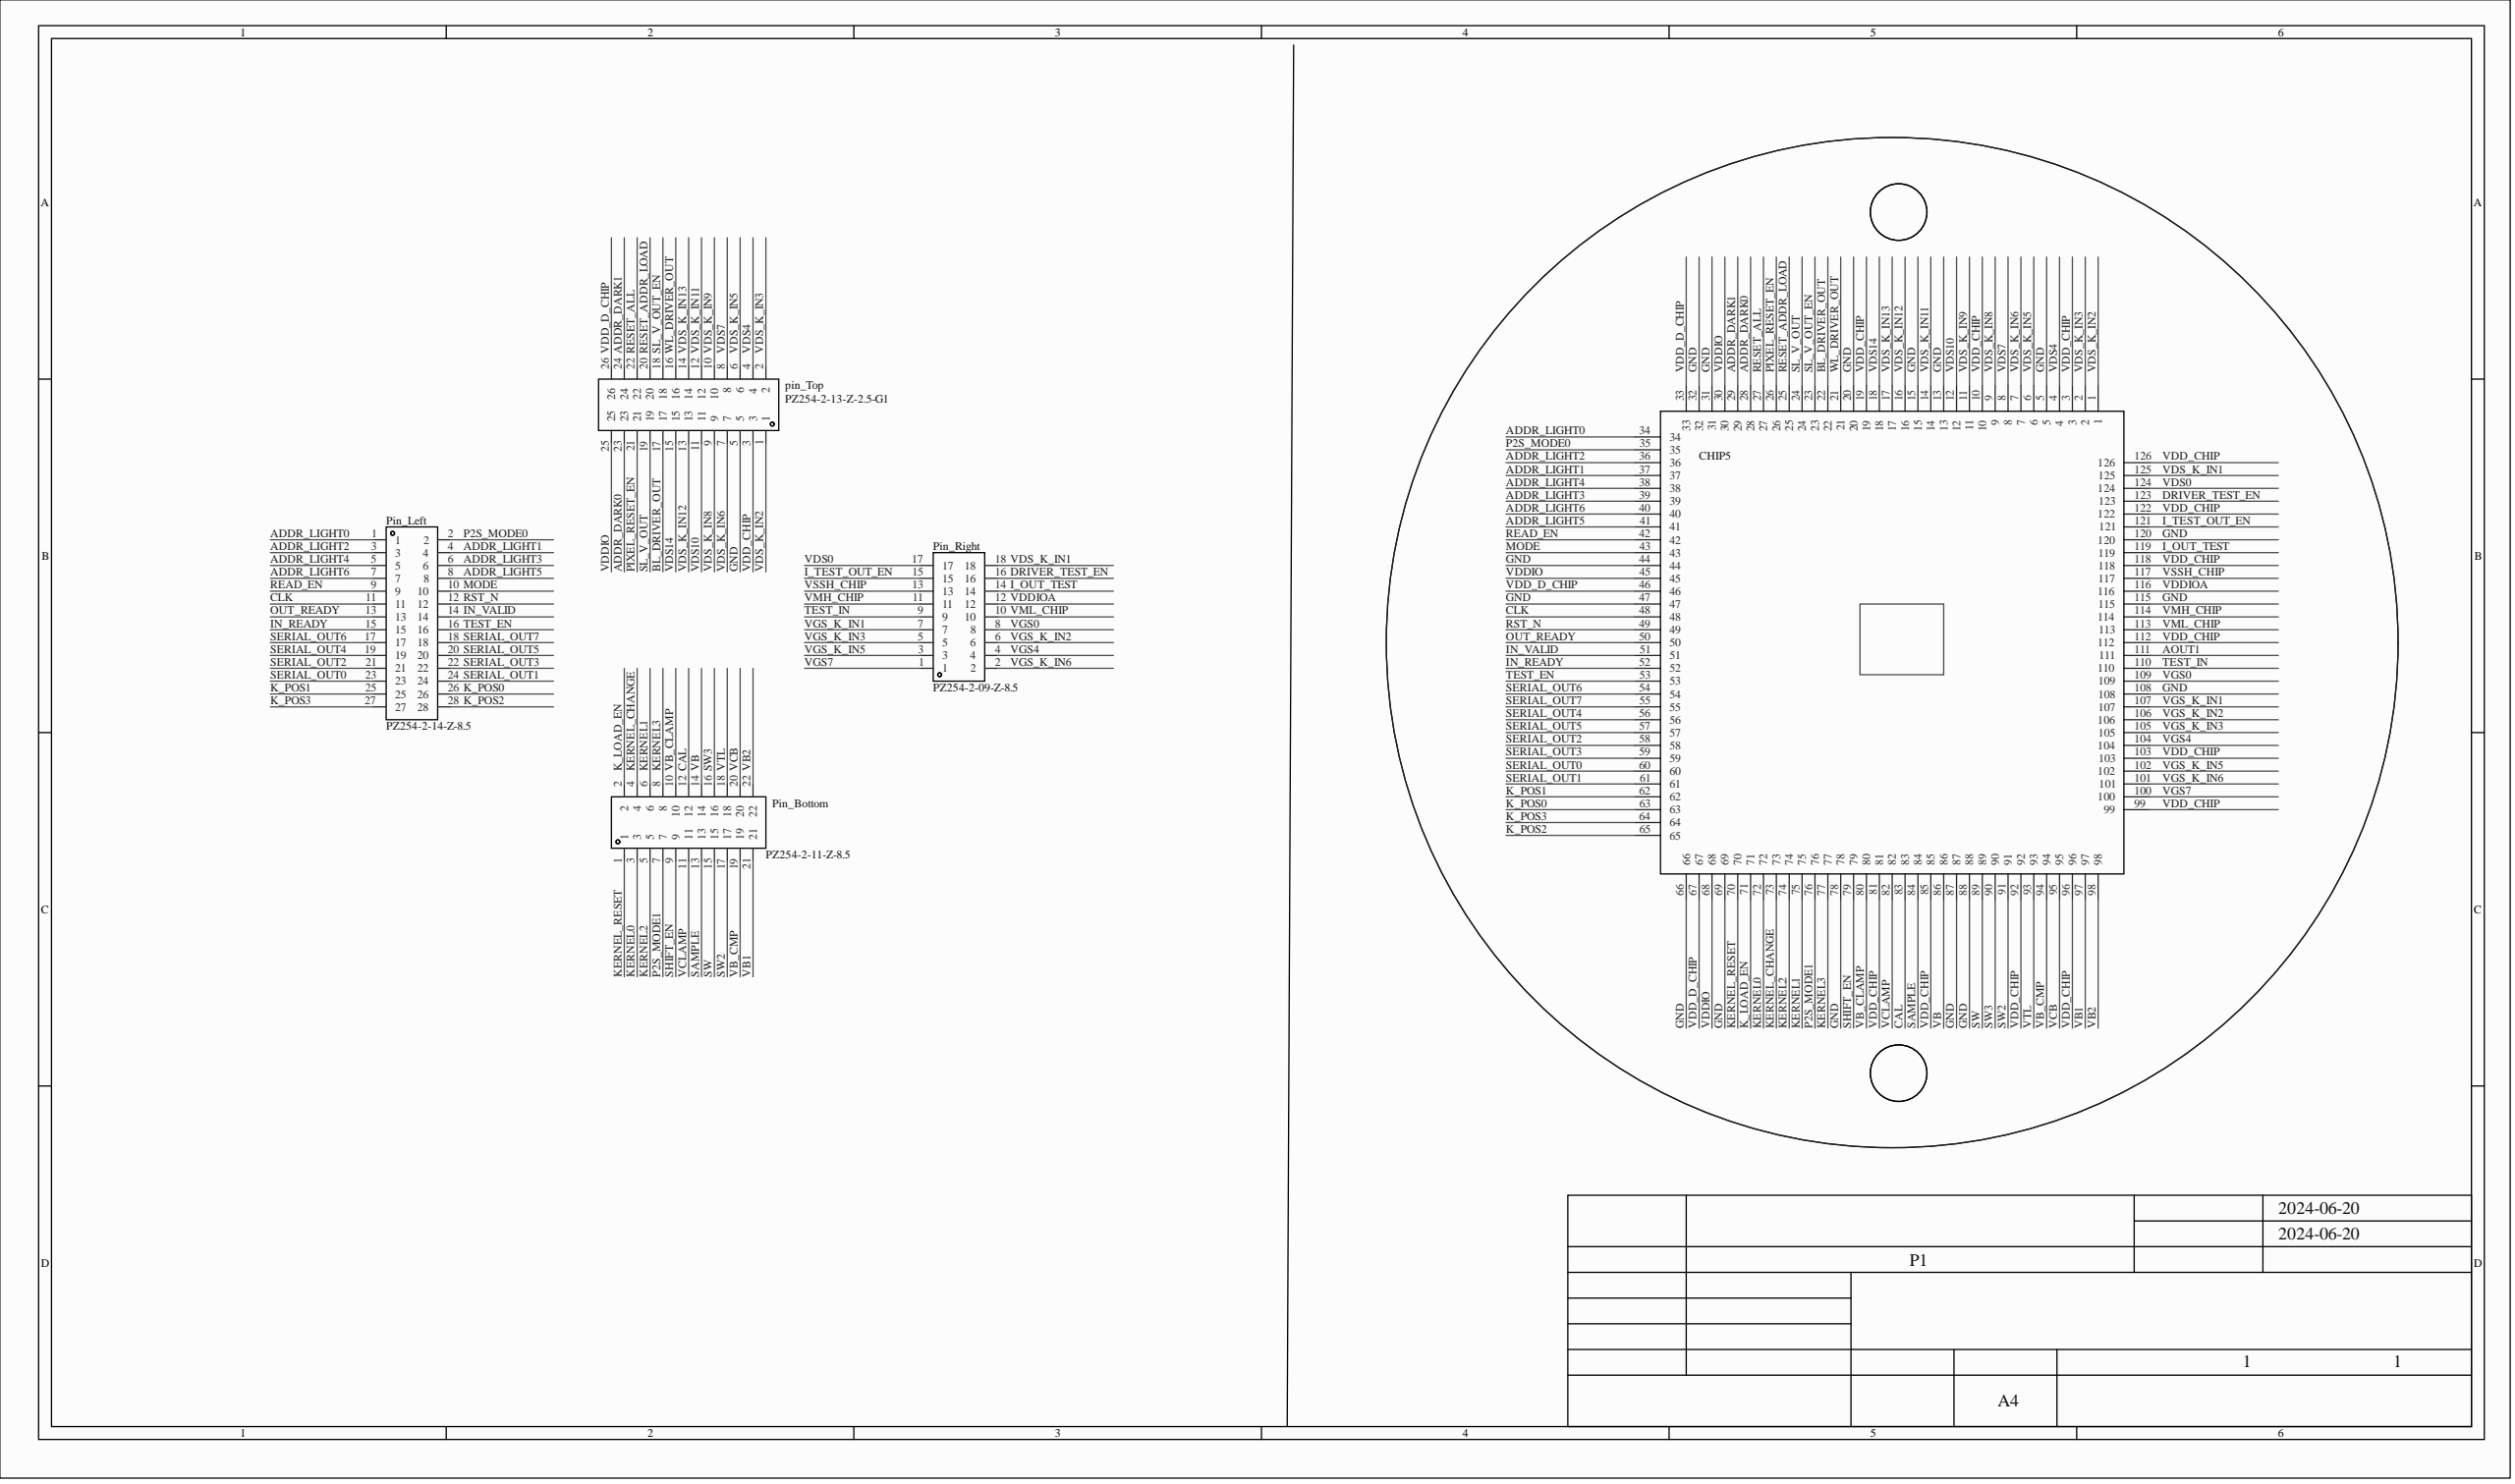Circuit board | Altium Designer | 5 parts | 94 nets
Bill of materials:
Comment,Description,Designator,Footprint,LibRef,Quantity
"chip5","","CHIP5","JSZ","chip5","1"
"PZ254-2-11-Z-8.5","","Pin_Bottom","HDR2.54-LI-2x11P","PZ254-2-11-Z-8.5","1"
"PZ254-2-14-Z-8.5","","Pin_Left","HDR2.54-LI-2x14P","PZ254-2-14-Z-8.5","1"
"PZ254-2-09-Z-8.5","","Pin_Right","HDR2.54-LI-2x9P","PZ254-2-09-Z-8.5","1"
"PZ254-2-13-Z-2.5-G1","","pin_Top","HDR2.54-LI-2x13P","PZ254-2-13-Z-2.5-G1","1"
Netlist (Protel format):
[
CHIP5
JSZ
chip5



]
[
Pin_Bottom
HDR2.54-LI-2x11P
PZ254-2-11-Z-8.5



]
[
Pin_Left
HDR2.54-LI-2x14P
PZ254-2-14-Z-8.5



]
[
Pin_Right
HDR2.54-LI-2x9P
PZ254-2-09-Z-8.5



]
[
pin_Top
HDR2.54-LI-2x13P
PZ254-2-13-Z-2.5-G1



]
(
WL_DRIVER_OUT
CHIP5-21
pin_Top-16
)
(
VTL
CHIP5-93
Pin_Bottom-18
)
(
VSSH_CHIP
CHIP5-117
Pin_Right-13
)
(
VML_CHIP
CHIP5-113
Pin_Right-10
)
(
VMH_CHIP
CHIP5-114
Pin_Right-11
)
(
VGS_K_IN6
CHIP5-101
Pin_Right-2
)
(
VGS_K_IN5
CHIP5-102
Pin_Right-3
)
(
VGS_K_IN3
CHIP5-105
Pin_Right-5
)
(
VGS_K_IN2
CHIP5-106
Pin_Right-6
)
(
VGS_K_IN1
CHIP5-107
Pin_Right-7
)
(
VGS7
CHIP5-100
Pin_Right-1
)
(
VGS4
CHIP5-104
Pin_Right-4
)
(
VGS0
CHIP5-109
Pin_Right-8
)
(
VDS_K_IN13
CHIP5-17
pin_Top-14
)
(
VDS_K_IN12
CHIP5-16
pin_Top-13
)
(
VDS_K_IN11
CHIP5-14
pin_Top-12
)
(
VDS_K_IN9
CHIP5-11
pin_Top-10
)
(
VDS_K_IN8
CHIP5-9
pin_Top-9
)
(
VDS_K_IN6
CHIP5-7
pin_Top-7
)
(
VDS_K_IN5
CHIP5-6
pin_Top-6
)
(
VDS_K_IN3
CHIP5-2
pin_Top-2
)
(
VDS_K_IN2
CHIP5-1
pin_Top-1
)
(
VDS_K_IN1
CHIP5-125
Pin_Right-18
)
(
VDS14
CHIP5-18
pin_Top-15
)
(
VDS10
CHIP5-12
pin_Top-11
)
(
VDS7
CHIP5-8
pin_Top-8
)
(
VDS4
CHIP5-4
pin_Top-4
)
(
VDS0
CHIP5-124
Pin_Right-17
)
(
VDDIOA
CHIP5-116
Pin_Right-12
)
(
VDDIO
CHIP5-30
CHIP5-45
CHIP5-68
pin_Top-25
)
(
VDD_D_CHIP
CHIP5-33
CHIP5-46
CHIP5-67
pin_Top-26
)
(
VDD_CHIP
CHIP5-3
CHIP5-10
CHIP5-19
CHIP5-81
CHIP5-85
CHIP5-92
CHIP5-96
CHIP5-99
CHIP5-103
CHIP5-112
CHIP5-118
CHIP5-122
CHIP5-126
pin_Top-3
)
(
VCLAMP
CHIP5-82
Pin_Bottom-11
)
(
VCB
CHIP5-95
Pin_Bottom-20
)
(
VB_CMP
CHIP5-94
Pin_Bottom-19
)
(
VB_CLAMP
CHIP5-80
Pin_Bottom-10
)
(
VB2
CHIP5-98
Pin_Bottom-22
)
(
VB1
CHIP5-97
Pin_Bottom-21
)
(
VB
CHIP5-86
Pin_Bottom-14
)
(
TEST_IN
CHIP5-110
Pin_Right-9
)
(
TEST_EN
CHIP5-53
Pin_Left-16
)
(
SW3
CHIP5-90
Pin_Bottom-16
)
(
SW2
CHIP5-91
Pin_Bottom-17
)
(
SW
CHIP5-89
Pin_Bottom-15
)
(
SL_V_OUT_EN
CHIP5-23
pin_Top-18
)
(
SL_V_OUT
CHIP5-24
pin_Top-19
)
(
SHIFT_EN
CHIP5-79
Pin_Bottom-9
)
(
SERIAL_OUT7
CHIP5-55
Pin_Left-18
)
(
SERIAL_OUT6
CHIP5-54
Pin_Left-17
)
(
SERIAL_OUT5
CHIP5-57
Pin_Left-20
)
(
SERIAL_OUT4
CHIP5-56
Pin_Left-19
)
(
SERIAL_OUT3
CHIP5-59
Pin_Left-22
)
(
SERIAL_OUT2
CHIP5-58
Pin_Left-21
)
(
SERIAL_OUT1
CHIP5-61
Pin_Left-24
)
(
SERIAL_OUT0
CHIP5-60
Pin_Left-23
)
(
SAMPLE
CHIP5-84
Pin_Bottom-13
)
(
RST_N
CHIP5-49
Pin_Left-12
)
(
RESET_ALL
CHIP5-27
pin_Top-22
)
(
RESET_ADDR_LOAD
CHIP5-25
pin_Top-20
)
(
READ_EN
CHIP5-42
Pin_Left-9
)
(
PIXEL_RESET_EN
CHIP5-26
pin_Top-21
)
(
P2S_MODE1
CHIP5-76
Pin_Bottom-7
)
(
P2S_MODE0
CHIP5-35
Pin_Left-2
)
(
OUT_READY
CHIP5-50
Pin_Left-13
)
(
MODE
CHIP5-43
Pin_Left-10
)
(
KERNEL_RESET
CHIP5-70
Pin_Bottom-1
)
(
KERNEL_CHANGE
CHIP5-73
Pin_Bottom-4
)
(
KERNEL3
CHIP5-77
Pin_Bottom-8
)
(
KERNEL2
CHIP5-74
Pin_Bottom-5
)
(
KERNEL1
CHIP5-75
Pin_Bottom-6
)
(
KERNEL0
CHIP5-72
Pin_Bottom-3
)
(
K_POS3
CHIP5-64
Pin_Left-27
)
(
K_POS2
CHIP5-65
Pin_Left-28
)
(
K_POS1
CHIP5-62
Pin_Left-25
)
(
K_POS0
CHIP5-63
Pin_Left-26
)
(
K_LOAD_EN
CHIP5-71
Pin_Bottom-2
)
(
IN_VALID
CHIP5-51
Pin_Left-14
)
(
IN_READY
CHIP5-52
Pin_Left-15
)
(
I_TEST_OUT_EN
CHIP5-121
Pin_Right-15
)
(
I_OUT_TEST
CHIP5-119
Pin_Right-14
)
(
GND
CHIP5-5
CHIP5-13
CHIP5-15
CHIP5-20
CHIP5-31
CHIP5-32
CHIP5-44
CHIP5-47
CHIP5-66
CHIP5-69
CHIP5-78
CHIP5-87
CHIP5-88
CHIP5-108
CHIP5-115
CHIP5-120
pin_Top-5
)
(
DRIVER_TEST_EN
CHIP5-123
Pin_Right-16
)
(
CLK
CHIP5-48
Pin_Left-11
)
(
CAL
CHIP5-83
Pin_Bottom-12
)
(
BL_DRIVER_OUT
CHIP5-22
pin_Top-17
)
(
ADDR_LIGHT6
CHIP5-40
Pin_Left-7
)
(
ADDR_LIGHT5
CHIP5-41
Pin_Left-8
)
(
ADDR_LIGHT4
CHIP5-38
Pin_Left-5
)
(
ADDR_LIGHT3
CHIP5-39
Pin_Left-6
)
(
ADDR_LIGHT2
CHIP5-36
Pin_Left-3
)
(
ADDR_LIGHT1
CHIP5-37
Pin_Left-4
)
(
ADDR_LIGHT0
CHIP5-34
Pin_Left-1
)
(
ADDR_DARK1
CHIP5-29
pin_Top-24
)
(
ADDR_DARK0
CHIP5-28
pin_Top-23
)